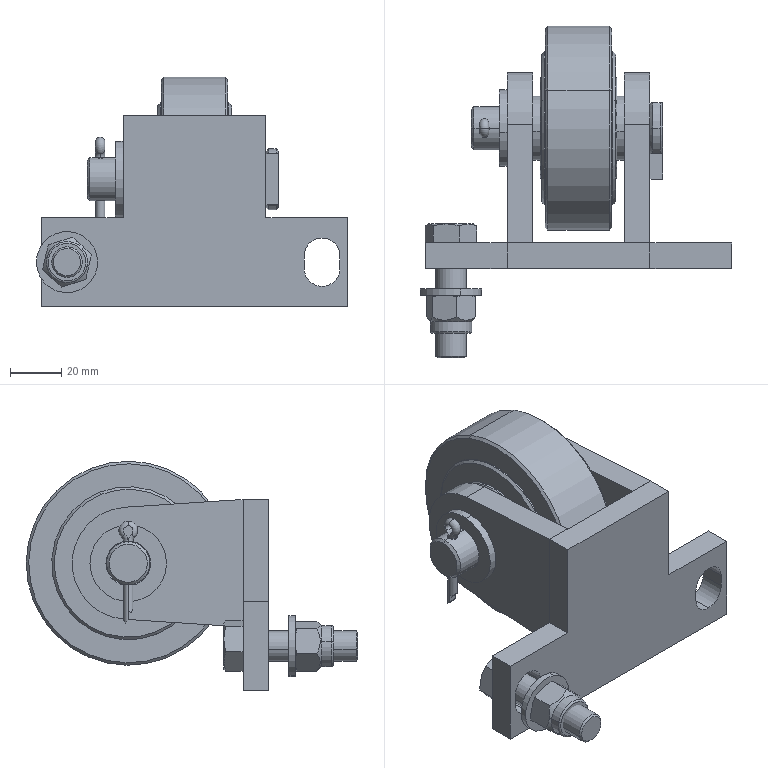Part | SolidWorks | features CompositeCurve 1 | 42 solids | 546 faces | box 122 x 130 x 90 mm | volume 267723 mm3 | cylinder 198 | plane 140 | sphere 104 | cone 52 | torus 52 | commonest cylinder face diameters 27.35 x46 29.65 x46 17 x14 60 x12 24.667 x8 32.333 x8